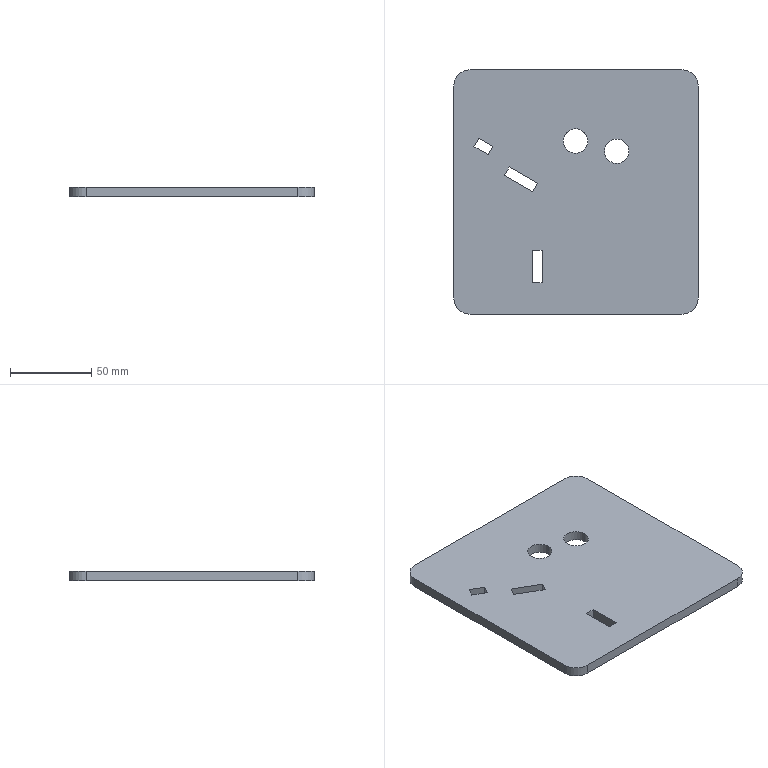Part | SolidWorks | features FlatPattern 1, SMBaseFlange 1, SheetMetal 1 | 1 solid | 26 faces | box 150 x 150 x 6 mm | volume 130564 mm3 | plane 18 | cylinder 8 | commonest cylinder face diameters 15 x4 20 x4
STEP:
#1=CARTESIAN_POINT('',(-26.981,-17.057,6.));
#2=VERTEX_POINT('',#1);
#3=CARTESIAN_POINT('',(-11.981,-17.057,6.));
#4=VERTEX_POINT('',#3);
#5=CARTESIAN_POINT('',(-19.481,-17.057,6.));
#6=DIRECTION('',(0.,0.,1.));
#7=DIRECTION('',(1.,0.,0.));
#8=AXIS2_PLACEMENT_3D('',#5,#6,#7);
#9=CIRCLE('',#8,7.5);
#10=EDGE_CURVE('',#2,#4,#9,.T.);
#11=ORIENTED_EDGE('',*,*,#10,.T.);
#12=CARTESIAN_POINT('',(-11.981,-17.057,0.));
#13=VERTEX_POINT('',#12);
#14=CARTESIAN_POINT('',(-11.981,-17.057,6.));
#15=DIRECTION('',(0.,0.,-1.));
#16=VECTOR('',#15,1000.);
#17=LINE('',#14,#16);
#18=EDGE_CURVE('',#4,#13,#17,.T.);
#19=ORIENTED_EDGE('',*,*,#18,.T.);
#20=CARTESIAN_POINT('',(-26.981,-17.057,0.));
#21=VERTEX_POINT('',#20);
#22=CARTESIAN_POINT('',(-19.481,-17.057,0.));
#23=DIRECTION('',(0.,0.,1.));
#24=DIRECTION('',(1.,0.,0.));
#25=AXIS2_PLACEMENT_3D('',#22,#23,#24);
#26=CIRCLE('',#25,7.5);
#27=EDGE_CURVE('',#21,#13,#26,.T.);
#28=ORIENTED_EDGE('',*,*,#27,.F.);
#29=CARTESIAN_POINT('',(-26.981,-17.057,6.));
#30=DIRECTION('',(0.,0.,-1.));
#31=VECTOR('',#30,1000.);
#32=LINE('',#29,#31);
#33=EDGE_CURVE('',#2,#21,#32,.T.);
#34=ORIENTED_EDGE('',*,*,#33,.F.);
#35=EDGE_LOOP('',(#11,#19,#28,#34));
#36=FACE_OUTER_BOUND('',#35,.T.);
#37=CARTESIAN_POINT('',(-19.481,-17.057,6.));
#38=DIRECTION('',(0.,0.,-1.));
#39=DIRECTION('',(-1.,0.,0.));
#40=AXIS2_PLACEMENT_3D('',#37,#38,#39);
#41=CYLINDRICAL_SURFACE('',#40,7.5);
#42=ADVANCED_FACE('',(#36),#41,.F.);
#43=CARTESIAN_POINT('',(-1.739,-23.292,6.));
#44=VERTEX_POINT('',#43);
#45=CARTESIAN_POINT('',(13.261,-23.292,6.));
#46=VERTEX_POINT('',#45);
#47=CARTESIAN_POINT('',(5.761,-23.292,6.));
#48=DIRECTION('',(0.,0.,1.));
#49=DIRECTION('',(1.,0.,0.));
#50=AXIS2_PLACEMENT_3D('',#47,#48,#49);
#51=CIRCLE('',#50,7.5);
#52=EDGE_CURVE('',#44,#46,#51,.T.);
#53=ORIENTED_EDGE('',*,*,#52,.T.);
#54=CARTESIAN_POINT('',(13.261,-23.292,0.));
#55=VERTEX_POINT('',#54);
#56=CARTESIAN_POINT('',(13.261,-23.292,6.));
#57=DIRECTION('',(0.,0.,-1.));
#58=VECTOR('',#57,1000.);
#59=LINE('',#56,#58);
#60=EDGE_CURVE('',#46,#55,#59,.T.);
#61=ORIENTED_EDGE('',*,*,#60,.T.);
#62=CARTESIAN_POINT('',(-1.739,-23.292,0.));
#63=VERTEX_POINT('',#62);
#64=CARTESIAN_POINT('',(5.761,-23.292,0.));
#65=DIRECTION('',(0.,0.,1.));
#66=DIRECTION('',(1.,0.,0.));
#67=AXIS2_PLACEMENT_3D('',#64,#65,#66);
#68=CIRCLE('',#67,7.5);
#69=EDGE_CURVE('',#63,#55,#68,.T.);
#70=ORIENTED_EDGE('',*,*,#69,.F.);
#71=CARTESIAN_POINT('',(-1.739,-23.292,6.));
#72=DIRECTION('',(0.,0.,-1.));
#73=VECTOR('',#72,1000.);
#74=LINE('',#71,#73);
#75=EDGE_CURVE('',#44,#63,#74,.T.);
#76=ORIENTED_EDGE('',*,*,#75,.F.);
#77=EDGE_LOOP('',(#53,#61,#70,#76));
#78=FACE_OUTER_BOUND('',#77,.T.);
#79=CARTESIAN_POINT('',(5.761,-23.292,6.));
#80=DIRECTION('',(0.,0.,-1.));
#81=DIRECTION('',(-1.,0.,0.));
#82=AXIS2_PLACEMENT_3D('',#79,#80,#81);
#83=CYLINDRICAL_SURFACE('',#82,7.5);
#84=ADVANCED_FACE('',(#78),#83,.F.);
#85=CARTESIAN_POINT('',(-45.869,-48.093,6.));
#86=VERTEX_POINT('',#85);
#87=CARTESIAN_POINT('',(-42.869,-42.897,6.));
#88=VERTEX_POINT('',#87);
#89=CARTESIAN_POINT('',(-45.869,-48.093,6.));
#90=DIRECTION('',(0.5,0.866,0.));
#91=VECTOR('',#90,1000.);
#92=LINE('',#89,#91);
#93=EDGE_CURVE('',#86,#88,#92,.T.);
#94=ORIENTED_EDGE('',*,*,#93,.F.);
#95=CARTESIAN_POINT('',(-63.19,-38.093,6.));
#96=VERTEX_POINT('',#95);
#97=CARTESIAN_POINT('',(-63.19,-38.093,6.));
#98=DIRECTION('',(0.866,-0.5,0.));
#99=VECTOR('',#98,1000.);
#100=LINE('',#97,#99);
#101=EDGE_CURVE('',#96,#86,#100,.T.);
#102=ORIENTED_EDGE('',*,*,#101,.F.);
#103=CARTESIAN_POINT('',(-60.19,-32.897,6.));
#104=VERTEX_POINT('',#103);
#105=CARTESIAN_POINT('',(-60.19,-32.897,6.));
#106=DIRECTION('',(-0.5,-0.866,0.));
#107=VECTOR('',#106,1000.);
#108=LINE('',#105,#107);
#109=EDGE_CURVE('',#104,#96,#108,.T.);
#110=ORIENTED_EDGE('',*,*,#109,.F.);
#111=CARTESIAN_POINT('',(-42.869,-42.897,6.));
#112=DIRECTION('',(-0.866,0.5,0.));
#113=VECTOR('',#112,1000.);
#114=LINE('',#111,#113);
#115=EDGE_CURVE('',#88,#104,#114,.T.);
#116=ORIENTED_EDGE('',*,*,#115,.F.);
#117=EDGE_LOOP('',(#94,#102,#110,#116));
#118=FACE_BOUND('',#117,.T.);
#119=ORIENTED_EDGE('',*,*,#10,.F.);
#120=CARTESIAN_POINT('',(-19.481,-17.057,6.));
#121=DIRECTION('',(0.,0.,1.));
#122=DIRECTION('',(1.,0.,0.));
#123=AXIS2_PLACEMENT_3D('',#120,#121,#122);
#124=CIRCLE('',#123,7.5);
#125=EDGE_CURVE('',#4,#2,#124,.T.);
#126=ORIENTED_EDGE('',*,*,#125,.F.);
#127=EDGE_LOOP('',(#119,#126));
#128=FACE_BOUND('',#127,.T.);
#129=ORIENTED_EDGE('',*,*,#52,.F.);
#130=CARTESIAN_POINT('',(5.761,-23.292,6.));
#131=DIRECTION('',(0.,0.,1.));
#132=DIRECTION('',(1.,0.,0.));
#133=AXIS2_PLACEMENT_3D('',#130,#131,#132);
#134=CIRCLE('',#133,7.5);
#135=EDGE_CURVE('',#46,#44,#134,.T.);
#136=ORIENTED_EDGE('',*,*,#135,.F.);
#137=EDGE_LOOP('',(#129,#136));
#138=FACE_BOUND('',#137,.T.);
#139=CARTESIAN_POINT('',(-84.239,26.708,6.));
#140=VERTEX_POINT('',#139);
#141=CARTESIAN_POINT('',(-94.239,16.708,6.));
#142=VERTEX_POINT('',#141);
#143=CARTESIAN_POINT('',(-84.239,16.708,6.));
#144=DIRECTION('',(0.,0.,1.));
#145=DIRECTION('',(-1.,0.,0.));
#146=AXIS2_PLACEMENT_3D('',#143,#144,#145);
#147=CIRCLE('',#146,10.);
#148=EDGE_CURVE('',#140,#142,#147,.T.);
#149=ORIENTED_EDGE('',*,*,#148,.T.);
#150=CARTESIAN_POINT('',(-94.239,-113.292,6.));
#151=VERTEX_POINT('',#150);
#152=CARTESIAN_POINT('',(-94.239,-113.292,6.));
#153=DIRECTION('',(0.,-1.,0.));
#154=VECTOR('',#153,1000.);
#155=LINE('',#152,#154);
#156=EDGE_CURVE('',#142,#151,#155,.T.);
#157=ORIENTED_EDGE('',*,*,#156,.T.);
#158=CARTESIAN_POINT('',(-84.239,-123.292,6.));
#159=VERTEX_POINT('',#158);
#160=CARTESIAN_POINT('',(-84.239,-113.292,6.));
#161=DIRECTION('',(0.,0.,1.));
#162=DIRECTION('',(-1.,0.,0.));
#163=AXIS2_PLACEMENT_3D('',#160,#161,#162);
#164=CIRCLE('',#163,10.);
#165=EDGE_CURVE('',#151,#159,#164,.T.);
#166=ORIENTED_EDGE('',*,*,#165,.T.);
#167=CARTESIAN_POINT('',(45.761,-123.292,6.));
#168=VERTEX_POINT('',#167);
#169=CARTESIAN_POINT('',(45.761,-123.292,6.));
#170=DIRECTION('',(1.,0.,0.));
#171=VECTOR('',#170,1000.);
#172=LINE('',#169,#171);
#173=EDGE_CURVE('',#159,#168,#172,.T.);
#174=ORIENTED_EDGE('',*,*,#173,.T.);
#175=CARTESIAN_POINT('',(55.761,-113.292,6.));
#176=VERTEX_POINT('',#175);
#177=CARTESIAN_POINT('',(45.761,-113.292,6.));
#178=DIRECTION('',(0.,0.,1.));
#179=DIRECTION('',(1.,0.,0.));
#180=AXIS2_PLACEMENT_3D('',#177,#178,#179);
#181=CIRCLE('',#180,10.);
#182=EDGE_CURVE('',#168,#176,#181,.T.);
#183=ORIENTED_EDGE('',*,*,#182,.T.);
#184=CARTESIAN_POINT('',(55.761,16.708,6.));
#185=VERTEX_POINT('',#184);
#186=CARTESIAN_POINT('',(55.761,16.708,6.));
#187=DIRECTION('',(0.,1.,0.));
#188=VECTOR('',#187,1000.);
#189=LINE('',#186,#188);
#190=EDGE_CURVE('',#176,#185,#189,.T.);
#191=ORIENTED_EDGE('',*,*,#190,.T.);
#192=CARTESIAN_POINT('',(45.761,26.708,6.));
#193=VERTEX_POINT('',#192);
#194=CARTESIAN_POINT('',(45.761,16.708,6.));
#195=DIRECTION('',(0.,0.,1.));
#196=DIRECTION('',(-1.,0.,0.));
#197=AXIS2_PLACEMENT_3D('',#194,#195,#196);
#198=CIRCLE('',#197,10.);
#199=EDGE_CURVE('',#185,#193,#198,.T.);
#200=ORIENTED_EDGE('',*,*,#199,.T.);
#201=CARTESIAN_POINT('',(-84.239,26.708,6.));
#202=DIRECTION('',(-1.,0.,0.));
#203=VECTOR('',#202,1000.);
#204=LINE('',#201,#203);
#205=EDGE_CURVE('',#193,#140,#204,.T.);
#206=ORIENTED_EDGE('',*,*,#205,.T.);
#207=EDGE_LOOP('',(#149,#157,#166,#174,#183,#191,#200,#206));
#208=FACE_OUTER_BOUND('',#207,.T.);
#209=CARTESIAN_POINT('',(-40.,-104.,6.));
#210=VERTEX_POINT('',#209);
#211=CARTESIAN_POINT('',(-40.,-84.,6.));
#212=VERTEX_POINT('',#211);
#213=CARTESIAN_POINT('',(-40.,-104.,6.));
#214=DIRECTION('',(0.,1.,0.));
#215=VECTOR('',#214,1000.);
#216=LINE('',#213,#215);
#217=EDGE_CURVE('',#210,#212,#216,.T.);
#218=ORIENTED_EDGE('',*,*,#217,.F.);
#219=CARTESIAN_POINT('',(-46.,-104.,6.));
#220=VERTEX_POINT('',#219);
#221=CARTESIAN_POINT('',(-46.,-104.,6.));
#222=DIRECTION('',(1.,0.,0.));
#223=VECTOR('',#222,1000.);
#224=LINE('',#221,#223);
#225=EDGE_CURVE('',#220,#210,#224,.T.);
#226=ORIENTED_EDGE('',*,*,#225,.F.);
#227=CARTESIAN_POINT('',(-46.,-84.,6.));
#228=VERTEX_POINT('',#227);
#229=CARTESIAN_POINT('',(-46.,-84.,6.));
#230=DIRECTION('',(0.,-1.,0.));
#231=VECTOR('',#230,1000.);
#232=LINE('',#229,#231);
#233=EDGE_CURVE('',#228,#220,#232,.T.);
#234=ORIENTED_EDGE('',*,*,#233,.F.);
#235=CARTESIAN_POINT('',(-40.,-84.,6.));
#236=DIRECTION('',(-1.,0.,0.));
#237=VECTOR('',#236,1000.);
#238=LINE('',#235,#237);
#239=EDGE_CURVE('',#212,#228,#238,.T.);
#240=ORIENTED_EDGE('',*,*,#239,.F.);
#241=EDGE_LOOP('',(#218,#226,#234,#240));
#242=FACE_BOUND('',#241,.T.);
#243=CARTESIAN_POINT('',(-78.84,-15.201,6.));
#244=VERTEX_POINT('',#243);
#245=CARTESIAN_POINT('',(-81.84,-20.397,6.));
#246=VERTEX_POINT('',#245);
#247=CARTESIAN_POINT('',(-81.84,-20.397,6.));
#248=DIRECTION('',(-0.5,-0.866,0.));
#249=VECTOR('',#248,1000.);
#250=LINE('',#247,#249);
#251=EDGE_CURVE('',#244,#246,#250,.T.);
#252=ORIENTED_EDGE('',*,*,#251,.F.);
#253=CARTESIAN_POINT('',(-70.18,-20.201,6.));
#254=VERTEX_POINT('',#253);
#255=CARTESIAN_POINT('',(-70.18,-20.201,6.));
#256=DIRECTION('',(-0.866,0.5,0.));
#257=VECTOR('',#256,1000.);
#258=LINE('',#255,#257);
#259=EDGE_CURVE('',#254,#244,#258,.T.);
#260=ORIENTED_EDGE('',*,*,#259,.F.);
#261=CARTESIAN_POINT('',(-73.18,-25.397,6.));
#262=VERTEX_POINT('',#261);
#263=CARTESIAN_POINT('',(-70.18,-20.201,6.));
#264=DIRECTION('',(0.5,0.866,0.));
#265=VECTOR('',#264,1000.);
#266=LINE('',#263,#265);
#267=EDGE_CURVE('',#262,#254,#266,.T.);
#268=ORIENTED_EDGE('',*,*,#267,.F.);
#269=CARTESIAN_POINT('',(-73.18,-25.397,6.));
#270=DIRECTION('',(0.866,-0.5,0.));
#271=VECTOR('',#270,1000.);
#272=LINE('',#269,#271);
#273=EDGE_CURVE('',#246,#262,#272,.T.);
#274=ORIENTED_EDGE('',*,*,#273,.F.);
#275=EDGE_LOOP('',(#252,#260,#268,#274));
#276=FACE_BOUND('',#275,.T.);
#277=CARTESIAN_POINT('',(-84.239,16.708,6.));
#278=DIRECTION('',(0.,0.,-1.));
#279=DIRECTION('',(-1.,0.,0.));
#280=AXIS2_PLACEMENT_3D('',#277,#278,#279);
#281=PLANE('',#280);
#282=ADVANCED_FACE('',(#118,#128,#138,#208,#242,#276),#281,.F.);
#283=ORIENTED_EDGE('',*,*,#69,.T.);
#284=CARTESIAN_POINT('',(5.761,-23.292,0.));
#285=DIRECTION('',(0.,0.,1.));
#286=DIRECTION('',(1.,0.,0.));
#287=AXIS2_PLACEMENT_3D('',#284,#285,#286);
#288=CIRCLE('',#287,7.5);
#289=EDGE_CURVE('',#55,#63,#288,.T.);
#290=ORIENTED_EDGE('',*,*,#289,.T.);
#291=EDGE_LOOP('',(#283,#290));
#292=FACE_BOUND('',#291,.T.);
#293=CARTESIAN_POINT('',(-84.239,26.708,0.));
#294=VERTEX_POINT('',#293);
#295=CARTESIAN_POINT('',(-94.239,16.708,0.));
#296=VERTEX_POINT('',#295);
#297=CARTESIAN_POINT('',(-84.239,16.708,0.));
#298=DIRECTION('',(0.,0.,1.));
#299=DIRECTION('',(-1.,0.,0.));
#300=AXIS2_PLACEMENT_3D('',#297,#298,#299);
#301=CIRCLE('',#300,10.);
#302=EDGE_CURVE('',#294,#296,#301,.T.);
#303=ORIENTED_EDGE('',*,*,#302,.F.);
#304=CARTESIAN_POINT('',(45.761,26.708,0.));
#305=VERTEX_POINT('',#304);
#306=CARTESIAN_POINT('',(-84.239,26.708,0.));
#307=DIRECTION('',(-1.,0.,0.));
#308=VECTOR('',#307,1000.);
#309=LINE('',#306,#308);
#310=EDGE_CURVE('',#305,#294,#309,.T.);
#311=ORIENTED_EDGE('',*,*,#310,.F.);
#312=CARTESIAN_POINT('',(55.761,16.708,0.));
#313=VERTEX_POINT('',#312);
#314=CARTESIAN_POINT('',(45.761,16.708,0.));
#315=DIRECTION('',(0.,0.,1.));
#316=DIRECTION('',(-1.,0.,0.));
#317=AXIS2_PLACEMENT_3D('',#314,#315,#316);
#318=CIRCLE('',#317,10.);
#319=EDGE_CURVE('',#313,#305,#318,.T.);
#320=ORIENTED_EDGE('',*,*,#319,.F.);
#321=CARTESIAN_POINT('',(55.761,-113.292,0.));
#322=VERTEX_POINT('',#321);
#323=CARTESIAN_POINT('',(55.761,16.708,0.));
#324=DIRECTION('',(0.,1.,0.));
#325=VECTOR('',#324,1000.);
#326=LINE('',#323,#325);
#327=EDGE_CURVE('',#322,#313,#326,.T.);
#328=ORIENTED_EDGE('',*,*,#327,.F.);
#329=CARTESIAN_POINT('',(45.761,-123.292,0.));
#330=VERTEX_POINT('',#329);
#331=CARTESIAN_POINT('',(45.761,-113.292,0.));
#332=DIRECTION('',(0.,0.,1.));
#333=DIRECTION('',(1.,0.,0.));
#334=AXIS2_PLACEMENT_3D('',#331,#332,#333);
#335=CIRCLE('',#334,10.);
#336=EDGE_CURVE('',#330,#322,#335,.T.);
#337=ORIENTED_EDGE('',*,*,#336,.F.);
#338=CARTESIAN_POINT('',(-84.239,-123.292,0.));
#339=VERTEX_POINT('',#338);
#340=CARTESIAN_POINT('',(45.761,-123.292,0.));
#341=DIRECTION('',(1.,0.,0.));
#342=VECTOR('',#341,1000.);
#343=LINE('',#340,#342);
#344=EDGE_CURVE('',#339,#330,#343,.T.);
#345=ORIENTED_EDGE('',*,*,#344,.F.);
#346=CARTESIAN_POINT('',(-94.239,-113.292,0.));
#347=VERTEX_POINT('',#346);
#348=CARTESIAN_POINT('',(-84.239,-113.292,0.));
#349=DIRECTION('',(0.,0.,1.));
#350=DIRECTION('',(-1.,0.,0.));
#351=AXIS2_PLACEMENT_3D('',#348,#349,#350);
#352=CIRCLE('',#351,10.);
#353=EDGE_CURVE('',#347,#339,#352,.T.);
#354=ORIENTED_EDGE('',*,*,#353,.F.);
#355=CARTESIAN_POINT('',(-94.239,-113.292,0.));
#356=DIRECTION('',(0.,-1.,0.));
#357=VECTOR('',#356,1000.);
#358=LINE('',#355,#357);
#359=EDGE_CURVE('',#296,#347,#358,.T.);
#360=ORIENTED_EDGE('',*,*,#359,.F.);
#361=EDGE_LOOP('',(#303,#311,#320,#328,#337,#345,#354,#360));
#362=FACE_OUTER_BOUND('',#361,.T.);
#363=ORIENTED_EDGE('',*,*,#27,.T.);
#364=CARTESIAN_POINT('',(-19.481,-17.057,0.));
#365=DIRECTION('',(0.,0.,1.));
#366=DIRECTION('',(1.,0.,0.));
#367=AXIS2_PLACEMENT_3D('',#364,#365,#366);
#368=CIRCLE('',#367,7.5);
#369=EDGE_CURVE('',#13,#21,#368,.T.);
#370=ORIENTED_EDGE('',*,*,#369,.T.);
#371=EDGE_LOOP('',(#363,#370));
#372=FACE_BOUND('',#371,.T.);
#373=CARTESIAN_POINT('',(-46.,-104.,0.));
#374=VERTEX_POINT('',#373);
#375=CARTESIAN_POINT('',(-40.,-104.,0.));
#376=VERTEX_POINT('',#375);
#377=CARTESIAN_POINT('',(-46.,-104.,0.));
#378=DIRECTION('',(1.,0.,0.));
#379=VECTOR('',#378,1000.);
#380=LINE('',#377,#379);
#381=EDGE_CURVE('',#374,#376,#380,.T.);
#382=ORIENTED_EDGE('',*,*,#381,.T.);
#383=CARTESIAN_POINT('',(-40.,-84.,0.));
#384=VERTEX_POINT('',#383);
#385=CARTESIAN_POINT('',(-40.,-104.,0.));
#386=DIRECTION('',(0.,1.,0.));
#387=VECTOR('',#386,1000.);
#388=LINE('',#385,#387);
#389=EDGE_CURVE('',#376,#384,#388,.T.);
#390=ORIENTED_EDGE('',*,*,#389,.T.);
#391=CARTESIAN_POINT('',(-46.,-84.,0.));
#392=VERTEX_POINT('',#391);
#393=CARTESIAN_POINT('',(-40.,-84.,0.));
#394=DIRECTION('',(-1.,0.,0.));
#395=VECTOR('',#394,1000.);
#396=LINE('',#393,#395);
#397=EDGE_CURVE('',#384,#392,#396,.T.);
#398=ORIENTED_EDGE('',*,*,#397,.T.);
#399=CARTESIAN_POINT('',(-46.,-84.,0.));
#400=DIRECTION('',(0.,-1.,0.));
#401=VECTOR('',#400,1000.);
#402=LINE('',#399,#401);
#403=EDGE_CURVE('',#392,#374,#402,.T.);
#404=ORIENTED_EDGE('',*,*,#403,.T.);
#405=EDGE_LOOP('',(#382,#390,#398,#404));
#406=FACE_BOUND('',#405,.T.);
#407=CARTESIAN_POINT('',(-63.19,-38.093,0.));
#408=VERTEX_POINT('',#407);
#409=CARTESIAN_POINT('',(-45.869,-48.093,0.));
#410=VERTEX_POINT('',#409);
#411=CARTESIAN_POINT('',(-63.19,-38.093,0.));
#412=DIRECTION('',(0.866,-0.5,0.));
#413=VECTOR('',#412,1000.);
#414=LINE('',#411,#413);
#415=EDGE_CURVE('',#408,#410,#414,.T.);
#416=ORIENTED_EDGE('',*,*,#415,.T.);
#417=CARTESIAN_POINT('',(-42.869,-42.897,0.));
#418=VERTEX_POINT('',#417);
#419=CARTESIAN_POINT('',(-45.869,-48.093,0.));
#420=DIRECTION('',(0.5,0.866,0.));
#421=VECTOR('',#420,1000.);
#422=LINE('',#419,#421);
#423=EDGE_CURVE('',#410,#418,#422,.T.);
#424=ORIENTED_EDGE('',*,*,#423,.T.);
#425=CARTESIAN_POINT('',(-60.19,-32.897,0.));
#426=VERTEX_POINT('',#425);
#427=CARTESIAN_POINT('',(-42.869,-42.897,0.));
#428=DIRECTION('',(-0.866,0.5,0.));
#429=VECTOR('',#428,1000.);
#430=LINE('',#427,#429);
#431=EDGE_CURVE('',#418,#426,#430,.T.);
#432=ORIENTED_EDGE('',*,*,#431,.T.);
#433=CARTESIAN_POINT('',(-60.19,-32.897,0.));
#434=DIRECTION('',(-0.5,-0.866,0.));
#435=VECTOR('',#434,1000.);
#436=LINE('',#433,#435);
#437=EDGE_CURVE('',#426,#408,#436,.T.);
#438=ORIENTED_EDGE('',*,*,#437,.T.);
#439=EDGE_LOOP('',(#416,#424,#432,#438));
#440=FACE_BOUND('',#439,.T.);
#441=CARTESIAN_POINT('',(-70.18,-20.201,0.));
#442=VERTEX_POINT('',#441);
#443=CARTESIAN_POINT('',(-78.84,-15.201,0.));
#444=VERTEX_POINT('',#443);
#445=CARTESIAN_POINT('',(-70.18,-20.201,0.));
#446=DIRECTION('',(-0.866,0.5,0.));
#447=VECTOR('',#446,1000.);
#448=LINE('',#445,#447);
#449=EDGE_CURVE('',#442,#444,#448,.T.);
#450=ORIENTED_EDGE('',*,*,#449,.T.);
#451=CARTESIAN_POINT('',(-81.84,-20.397,0.));
#452=VERTEX_POINT('',#451);
#453=CARTESIAN_POINT('',(-81.84,-20.397,0.));
#454=DIRECTION('',(-0.5,-0.866,0.));
#455=VECTOR('',#454,1000.);
#456=LINE('',#453,#455);
#457=EDGE_CURVE('',#444,#452,#456,.T.);
#458=ORIENTED_EDGE('',*,*,#457,.T.);
#459=CARTESIAN_POINT('',(-73.18,-25.397,0.));
#460=VERTEX_POINT('',#459);
#461=CARTESIAN_POINT('',(-73.18,-25.397,0.));
#462=DIRECTION('',(0.866,-0.5,0.));
#463=VECTOR('',#462,1000.);
#464=LINE('',#461,#463);
#465=EDGE_CURVE('',#452,#460,#464,.T.);
#466=ORIENTED_EDGE('',*,*,#465,.T.);
#467=CARTESIAN_POINT('',(-70.18,-20.201,0.));
#468=DIRECTION('',(0.5,0.866,0.));
#469=VECTOR('',#468,1000.);
#470=LINE('',#467,#469);
#471=EDGE_CURVE('',#460,#442,#470,.T.);
#472=ORIENTED_EDGE('',*,*,#471,.T.);
#473=EDGE_LOOP('',(#450,#458,#466,#472));
#474=FACE_BOUND('',#473,.T.);
#475=CARTESIAN_POINT('',(-84.239,16.708,0.));
#476=DIRECTION('',(0.,0.,-1.));
#477=DIRECTION('',(-1.,0.,0.));
#478=AXIS2_PLACEMENT_3D('',#475,#476,#477);
#479=PLANE('',#478);
#480=ADVANCED_FACE('',(#292,#362,#372,#406,#440,#474),#479,.T.);
#481=ORIENTED_EDGE('',*,*,#302,.T.);
#482=CARTESIAN_POINT('',(-94.239,16.708,6.));
#483=DIRECTION('',(0.,0.,-1.));
#484=VECTOR('',#483,1000.);
#485=LINE('',#482,#484);
#486=EDGE_CURVE('',#142,#296,#485,.T.);
#487=ORIENTED_EDGE('',*,*,#486,.F.);
#488=ORIENTED_EDGE('',*,*,#148,.F.);
#489=CARTESIAN_POINT('',(-84.239,26.708,6.));
#490=DIRECTION('',(0.,0.,-1.));
#491=VECTOR('',#490,1000.);
#492=LINE('',#489,#491);
#493=EDGE_CURVE('',#140,#294,#492,.T.);
#494=ORIENTED_EDGE('',*,*,#493,.T.);
#495=EDGE_LOOP('',(#481,#487,#488,#494));
#496=FACE_OUTER_BOUND('',#495,.T.);
#497=CARTESIAN_POINT('',(-84.239,16.708,6.));
#498=DIRECTION('',(0.,0.,-1.));
#499=DIRECTION('',(-1.,0.,0.));
#500=AXIS2_PLACEMENT_3D('',#497,#498,#499);
#501=CYLINDRICAL_SURFACE('',#500,10.);
#502=ADVANCED_FACE('',(#496),#501,.T.);
#503=ORIENTED_EDGE('',*,*,#359,.T.);
#504=CARTESIAN_POINT('',(-94.239,-113.292,6.));
#505=DIRECTION('',(0.,0.,-1.));
#506=VECTOR('',#505,1000.);
#507=LINE('',#504,#506);
#508=EDGE_CURVE('',#151,#347,#507,.T.);
#509=ORIENTED_EDGE('',*,*,#508,.F.);
#510=ORIENTED_EDGE('',*,*,#156,.F.);
#511=ORIENTED_EDGE('',*,*,#486,.T.);
#512=EDGE_LOOP('',(#503,#509,#510,#511));
#513=FACE_OUTER_BOUND('',#512,.T.);
#514=CARTESIAN_POINT('',(-94.239,-113.292,6.));
#515=DIRECTION('',(1.,0.,0.));
#516=DIRECTION('',(0.,1.,0.));
#517=AXIS2_PLACEMENT_3D('',#514,#515,#516);
#518=PLANE('',#517);
#519=ADVANCED_FACE('',(#513),#518,.F.);
#520=ORIENTED_EDGE('',*,*,#353,.T.);
#521=CARTESIAN_POINT('',(-84.239,-123.292,6.));
#522=DIRECTION('',(0.,0.,-1.));
#523=VECTOR('',#522,1000.);
#524=LINE('',#521,#523);
#525=EDGE_CURVE('',#159,#339,#524,.T.);
#526=ORIENTED_EDGE('',*,*,#525,.F.);
#527=ORIENTED_EDGE('',*,*,#165,.F.);
#528=ORIENTED_EDGE('',*,*,#508,.T.);
#529=EDGE_LOOP('',(#520,#526,#527,#528));
#530=FACE_OUTER_BOUND('',#529,.T.);
#531=CARTESIAN_POINT('',(-84.239,-113.292,6.));
#532=DIRECTION('',(0.,0.,-1.));
#533=DIRECTION('',(-1.,0.,0.));
#534=AXIS2_PLACEMENT_3D('',#531,#532,#533);
#535=CYLINDRICAL_SURFACE('',#534,10.);
#536=ADVANCED_FACE('',(#530),#535,.T.);
#537=ORIENTED_EDGE('',*,*,#344,.T.);
#538=CARTESIAN_POINT('',(45.761,-123.292,6.));
#539=DIRECTION('',(0.,0.,-1.));
#540=VECTOR('',#539,1000.);
#541=LINE('',#538,#540);
#542=EDGE_CURVE('',#168,#330,#541,.T.);
#543=ORIENTED_EDGE('',*,*,#542,.F.);
#544=ORIENTED_EDGE('',*,*,#173,.F.);
#545=ORIENTED_EDGE('',*,*,#525,.T.);
#546=EDGE_LOOP('',(#537,#543,#544,#545));
#547=FACE_OUTER_BOUND('',#546,.T.);
#548=CARTESIAN_POINT('',(45.761,-123.292,6.));
#549=DIRECTION('',(0.,1.,0.));
#550=DIRECTION('',(-1.,0.,0.));
#551=AXIS2_PLACEMENT_3D('',#548,#549,#550);
#552=PLANE('',#551);
#553=ADVANCED_FACE('',(#547),#552,.F.);
#554=ORIENTED_EDGE('',*,*,#336,.T.);
#555=CARTESIAN_POINT('',(55.761,-113.292,6.));
#556=DIRECTION('',(0.,0.,-1.));
#557=VECTOR('',#556,1000.);
#558=LINE('',#555,#557);
#559=EDGE_CURVE('',#176,#322,#558,.T.);
#560=ORIENTED_EDGE('',*,*,#559,.F.);
#561=ORIENTED_EDGE('',*,*,#182,.F.);
#562=ORIENTED_EDGE('',*,*,#542,.T.);
#563=EDGE_LOOP('',(#554,#560,#561,#562));
#564=FACE_OUTER_BOUND('',#563,.T.);
#565=CARTESIAN_POINT('',(45.761,-113.292,6.));
#566=DIRECTION('',(0.,0.,-1.));
#567=DIRECTION('',(-1.,0.,0.));
#568=AXIS2_PLACEMENT_3D('',#565,#566,#567);
#569=CYLINDRICAL_SURFACE('',#568,10.);
#570=ADVANCED_FACE('',(#564),#569,.T.);
#571=ORIENTED_EDGE('',*,*,#327,.T.);
#572=CARTESIAN_POINT('',(55.761,16.708,6.));
#573=DIRECTION('',(0.,0.,-1.));
#574=VECTOR('',#573,1000.);
#575=LINE('',#572,#574);
#576=EDGE_CURVE('',#185,#313,#575,.T.);
#577=ORIENTED_EDGE('',*,*,#576,.F.);
#578=ORIENTED_EDGE('',*,*,#190,.F.);
#579=ORIENTED_EDGE('',*,*,#559,.T.);
#580=EDGE_LOOP('',(#571,#577,#578,#579));
#581=FACE_OUTER_BOUND('',#580,.T.);
#582=CARTESIAN_POINT('',(55.761,16.708,6.));
#583=DIRECTION('',(-1.,0.,0.));
#584=DIRECTION('',(0.,-1.,0.));
#585=AXIS2_PLACEMENT_3D('',#582,#583,#584);
#586=PLANE('',#585);
#587=ADVANCED_FACE('',(#581),#586,.F.);
#588=ORIENTED_EDGE('',*,*,#319,.T.);
#589=CARTESIAN_POINT('',(45.761,26.708,6.));
#590=DIRECTION('',(0.,0.,-1.));
#591=VECTOR('',#590,1000.);
#592=LINE('',#589,#591);
#593=EDGE_CURVE('',#193,#305,#592,.T.);
#594=ORIENTED_EDGE('',*,*,#593,.F.);
#595=ORIENTED_EDGE('',*,*,#199,.F.);
#596=ORIENTED_EDGE('',*,*,#576,.T.);
#597=EDGE_LOOP('',(#588,#594,#595,#596));
#598=FACE_OUTER_BOUND('',#597,.T.);
#599=CARTESIAN_POINT('',(45.761,16.708,6.));
#600=DIRECTION('',(0.,0.,-1.));
#601=DIRECTION('',(-1.,0.,0.));
#602=AXIS2_PLACEMENT_3D('',#599,#600,#601);
#603=CYLINDRICAL_SURFACE('',#602,10.);
#604=ADVANCED_FACE('',(#598),#603,.T.);
#605=ORIENTED_EDGE('',*,*,#310,.T.);
#606=ORIENTED_EDGE('',*,*,#493,.F.);
#607=ORIENTED_EDGE('',*,*,#205,.F.);
#608=ORIENTED_EDGE('',*,*,#593,.T.);
#609=EDGE_LOOP('',(#605,#606,#607,#608));
#610=FACE_OUTER_BOUND('',#609,.T.);
#611=CARTESIAN_POINT('',(-84.239,26.708,6.));
#612=DIRECTION('',(0.,-1.,0.));
#613=DIRECTION('',(0.,0.,-1.));
#614=AXIS2_PLACEMENT_3D('',#611,#612,#613);
#615=PLANE('',#614);
#616=ADVANCED_FACE('',(#610),#615,.F.);
#617=ORIENTED_EDGE('',*,*,#60,.F.);
#618=ORIENTED_EDGE('',*,*,#135,.T.);
#619=ORIENTED_EDGE('',*,*,#75,.T.);
#620=ORIENTED_EDGE('',*,*,#289,.F.);
#621=EDGE_LOOP('',(#617,#618,#619,#620));
#622=FACE_OUTER_BOUND('',#621,.T.);
#623=CARTESIAN_POINT('',(5.761,-23.292,6.));
#624=DIRECTION('',(0.,0.,-1.));
#625=DIRECTION('',(-1.,0.,0.));
#626=AXIS2_PLACEMENT_3D('',#623,#624,#625);
#627=CYLINDRICAL_SURFACE('',#626,7.5);
#628=ADVANCED_FACE('',(#622),#627,.F.);
#629=ORIENTED_EDGE('',*,*,#18,.F.);
#630=ORIENTED_EDGE('',*,*,#125,.T.);
#631=ORIENTED_EDGE('',*,*,#33,.T.);
#632=ORIENTED_EDGE('',*,*,#369,.F.);
#633=EDGE_LOOP('',(#629,#630,#631,#632));
#634=FACE_OUTER_BOUND('',#633,.T.);
#635=CARTESIAN_POINT('',(-19.481,-17.057,6.));
#636=DIRECTION('',(0.,0.,-1.));
#637=DIRECTION('',(-1.,0.,0.));
#638=AXIS2_PLACEMENT_3D('',#635,#636,#637);
#639=CYLINDRICAL_SURFACE('',#638,7.5);
#640=ADVANCED_FACE('',(#634),#639,.F.);
#641=ORIENTED_EDGE('',*,*,#389,.F.);
#642=CARTESIAN_POINT('',(-40.,-104.,6.));
#643=DIRECTION('',(0.,0.,-1.));
#644=VECTOR('',#643,1000.);
#645=LINE('',#642,#644);
#646=EDGE_CURVE('',#210,#376,#645,.T.);
#647=ORIENTED_EDGE('',*,*,#646,.F.);
#648=ORIENTED_EDGE('',*,*,#217,.T.);
#649=CARTESIAN_POINT('',(-40.,-84.,6.));
#650=DIRECTION('',(0.,0.,-1.));
#651=VECTOR('',#650,1000.);
#652=LINE('',#649,#651);
#653=EDGE_CURVE('',#212,#384,#652,.T.);
#654=ORIENTED_EDGE('',*,*,#653,.T.);
#655=EDGE_LOOP('',(#641,#647,#648,#654));
#656=FACE_OUTER_BOUND('',#655,.T.);
#657=CARTESIAN_POINT('',(-40.,-104.,6.));
#658=DIRECTION('',(-1.,0.,0.));
#659=DIRECTION('',(0.,0.,1.));
#660=AXIS2_PLACEMENT_3D('',#657,#658,#659);
#661=PLANE('',#660);
#662=ADVANCED_FACE('',(#656),#661,.T.);
#663=ORIENTED_EDGE('',*,*,#397,.F.);
#664=ORIENTED_EDGE('',*,*,#653,.F.);
#665=ORIENTED_EDGE('',*,*,#239,.T.);
#666=CARTESIAN_POINT('',(-46.,-84.,6.));
#667=DIRECTION('',(0.,0.,-1.));
#668=VECTOR('',#667,1000.);
#669=LINE('',#666,#668);
#670=EDGE_CURVE('',#228,#392,#669,.T.);
#671=ORIENTED_EDGE('',*,*,#670,.T.);
#672=EDGE_LOOP('',(#663,#664,#665,#671));
#673=FACE_OUTER_BOUND('',#672,.T.);
#674=CARTESIAN_POINT('',(-40.,-84.,6.));
#675=DIRECTION('',(0.,-1.,0.));
#676=DIRECTION('',(0.,0.,-1.));
#677=AXIS2_PLACEMENT_3D('',#674,#675,#676);
#678=PLANE('',#677);
#679=ADVANCED_FACE('',(#673),#678,.T.);
#680=ORIENTED_EDGE('',*,*,#403,.F.);
#681=ORIENTED_EDGE('',*,*,#670,.F.);
#682=ORIENTED_EDGE('',*,*,#233,.T.);
#683=CARTESIAN_POINT('',(-46.,-104.,6.));
#684=DIRECTION('',(0.,0.,-1.));
#685=VECTOR('',#684,1000.);
#686=LINE('',#683,#685);
#687=EDGE_CURVE('',#220,#374,#686,.T.);
#688=ORIENTED_EDGE('',*,*,#687,.T.);
#689=EDGE_LOOP('',(#680,#681,#682,#688));
#690=FACE_OUTER_BOUND('',#689,.T.);
#691=CARTESIAN_POINT('',(-46.,-84.,6.));
#692=DIRECTION('',(1.,0.,0.));
#693=DIRECTION('',(0.,0.,-1.));
#694=AXIS2_PLACEMENT_3D('',#691,#692,#693);
#695=PLANE('',#694);
#696=ADVANCED_FACE('',(#690),#695,.T.);
#697=ORIENTED_EDGE('',*,*,#381,.F.);
#698=ORIENTED_EDGE('',*,*,#687,.F.);
#699=ORIENTED_EDGE('',*,*,#225,.T.);
#700=ORIENTED_EDGE('',*,*,#646,.T.);
#701=EDGE_LOOP('',(#697,#698,#699,#700));
#702=FACE_OUTER_BOUND('',#701,.T.);
#703=CARTESIAN_POINT('',(-46.,-104.,6.));
#704=DIRECTION('',(0.,1.,0.));
#705=DIRECTION('',(0.,0.,1.));
#706=AXIS2_PLACEMENT_3D('',#703,#704,#705);
#707=PLANE('',#706);
#708=ADVANCED_FACE('',(#702),#707,.T.);
#709=ORIENTED_EDGE('',*,*,#423,.F.);
#710=CARTESIAN_POINT('',(-45.869,-48.093,6.));
#711=DIRECTION('',(0.,0.,-1.));
#712=VECTOR('',#711,1000.);
#713=LINE('',#710,#712);
#714=EDGE_CURVE('',#86,#410,#713,.T.);
#715=ORIENTED_EDGE('',*,*,#714,.F.);
#716=ORIENTED_EDGE('',*,*,#93,.T.);
#717=CARTESIAN_POINT('',(-42.869,-42.897,6.));
#718=DIRECTION('',(0.,0.,-1.));
#719=VECTOR('',#718,1000.);
#720=LINE('',#717,#719);
#721=EDGE_CURVE('',#88,#418,#720,.T.);
#722=ORIENTED_EDGE('',*,*,#721,.T.);
#723=EDGE_LOOP('',(#709,#715,#716,#722));
#724=FACE_OUTER_BOUND('',#723,.T.);
#725=CARTESIAN_POINT('',(-45.869,-48.093,6.));
#726=DIRECTION('',(-0.866,0.5,0.));
#727=DIRECTION('',(-0.5,-0.866,0.));
#728=AXIS2_PLACEMENT_3D('',#725,#726,#727);
#729=PLANE('',#728);
#730=ADVANCED_FACE('',(#724),#729,.T.);
#731=ORIENTED_EDGE('',*,*,#431,.F.);
#732=ORIENTED_EDGE('',*,*,#721,.F.);
#733=ORIENTED_EDGE('',*,*,#115,.T.);
#734=CARTESIAN_POINT('',(-60.19,-32.897,6.));
#735=DIRECTION('',(0.,0.,-1.));
#736=VECTOR('',#735,1000.);
#737=LINE('',#734,#736);
#738=EDGE_CURVE('',#104,#426,#737,.T.);
#739=ORIENTED_EDGE('',*,*,#738,.T.);
#740=EDGE_LOOP('',(#731,#732,#733,#739));
#741=FACE_OUTER_BOUND('',#740,.T.);
#742=CARTESIAN_POINT('',(-42.869,-42.897,6.));
#743=DIRECTION('',(-0.5,-0.866,0.));
#744=DIRECTION('',(0.866,-0.5,0.));
#745=AXIS2_PLACEMENT_3D('',#742,#743,#744);
#746=PLANE('',#745);
#747=ADVANCED_FACE('',(#741),#746,.T.);
#748=ORIENTED_EDGE('',*,*,#437,.F.);
#749=ORIENTED_EDGE('',*,*,#738,.F.);
#750=ORIENTED_EDGE('',*,*,#109,.T.);
#751=CARTESIAN_POINT('',(-63.19,-38.093,6.));
#752=DIRECTION('',(0.,0.,-1.));
#753=VECTOR('',#752,1000.);
#754=LINE('',#751,#753);
#755=EDGE_CURVE('',#96,#408,#754,.T.);
#756=ORIENTED_EDGE('',*,*,#755,.T.);
#757=EDGE_LOOP('',(#748,#749,#750,#756));
#758=FACE_OUTER_BOUND('',#757,.T.);
#759=CARTESIAN_POINT('',(-60.19,-32.897,6.));
#760=DIRECTION('',(0.866,-0.5,0.));
#761=DIRECTION('',(0.5,0.866,0.));
#762=AXIS2_PLACEMENT_3D('',#759,#760,#761);
#763=PLANE('',#762);
#764=ADVANCED_FACE('',(#758),#763,.T.);
#765=ORIENTED_EDGE('',*,*,#415,.F.);
#766=ORIENTED_EDGE('',*,*,#755,.F.);
#767=ORIENTED_EDGE('',*,*,#101,.T.);
#768=ORIENTED_EDGE('',*,*,#714,.T.);
#769=EDGE_LOOP('',(#765,#766,#767,#768));
#770=FACE_OUTER_BOUND('',#769,.T.);
#771=CARTESIAN_POINT('',(-63.19,-38.093,6.));
#772=DIRECTION('',(0.5,0.866,0.));
#773=DIRECTION('',(-0.866,0.5,0.));
#774=AXIS2_PLACEMENT_3D('',#771,#772,#773);
#775=PLANE('',#774);
#776=ADVANCED_FACE('',(#770),#775,.T.);
#777=ORIENTED_EDGE('',*,*,#457,.F.);
#778=CARTESIAN_POINT('',(-78.84,-15.201,6.));
#779=DIRECTION('',(0.,0.,-1.));
#780=VECTOR('',#779,1000.);
#781=LINE('',#778,#780);
#782=EDGE_CURVE('',#244,#444,#781,.T.);
#783=ORIENTED_EDGE('',*,*,#782,.F.);
#784=ORIENTED_EDGE('',*,*,#251,.T.);
#785=CARTESIAN_POINT('',(-81.84,-20.397,6.));
#786=DIRECTION('',(0.,0.,-1.));
#787=VECTOR('',#786,1000.);
#788=LINE('',#785,#787);
#789=EDGE_CURVE('',#246,#452,#788,.T.);
#790=ORIENTED_EDGE('',*,*,#789,.T.);
#791=EDGE_LOOP('',(#777,#783,#784,#790));
#792=FACE_OUTER_BOUND('',#791,.T.);
#793=CARTESIAN_POINT('',(-81.84,-20.397,6.));
#794=DIRECTION('',(0.866,-0.5,0.));
#795=DIRECTION('',(0.5,0.866,0.));
#796=AXIS2_PLACEMENT_3D('',#793,#794,#795);
#797=PLANE('',#796);
#798=ADVANCED_FACE('',(#792),#797,.T.);
#799=ORIENTED_EDGE('',*,*,#465,.F.);
#800=ORIENTED_EDGE('',*,*,#789,.F.);
#801=ORIENTED_EDGE('',*,*,#273,.T.);
#802=CARTESIAN_POINT('',(-73.18,-25.397,6.));
#803=DIRECTION('',(0.,0.,-1.));
#804=VECTOR('',#803,1000.);
#805=LINE('',#802,#804);
#806=EDGE_CURVE('',#262,#460,#805,.T.);
#807=ORIENTED_EDGE('',*,*,#806,.T.);
#808=EDGE_LOOP('',(#799,#800,#801,#807));
#809=FACE_OUTER_BOUND('',#808,.T.);
#810=CARTESIAN_POINT('',(-73.18,-25.397,6.));
#811=DIRECTION('',(0.5,0.866,0.));
#812=DIRECTION('',(-0.866,0.5,0.));
#813=AXIS2_PLACEMENT_3D('',#810,#811,#812);
#814=PLANE('',#813);
#815=ADVANCED_FACE('',(#809),#814,.T.);
#816=ORIENTED_EDGE('',*,*,#471,.F.);
#817=ORIENTED_EDGE('',*,*,#806,.F.);
#818=ORIENTED_EDGE('',*,*,#267,.T.);
#819=CARTESIAN_POINT('',(-70.18,-20.201,6.));
#820=DIRECTION('',(0.,0.,-1.));
#821=VECTOR('',#820,1000.);
#822=LINE('',#819,#821);
#823=EDGE_CURVE('',#254,#442,#822,.T.);
#824=ORIENTED_EDGE('',*,*,#823,.T.);
#825=EDGE_LOOP('',(#816,#817,#818,#824));
#826=FACE_OUTER_BOUND('',#825,.T.);
#827=CARTESIAN_POINT('',(-70.18,-20.201,6.));
#828=DIRECTION('',(-0.866,0.5,0.));
#829=DIRECTION('',(-0.5,-0.866,0.));
#830=AXIS2_PLACEMENT_3D('',#827,#828,#829);
#831=PLANE('',#830);
#832=ADVANCED_FACE('',(#826),#831,.T.);
#833=ORIENTED_EDGE('',*,*,#449,.F.);
#834=ORIENTED_EDGE('',*,*,#823,.F.);
#835=ORIENTED_EDGE('',*,*,#259,.T.);
#836=ORIENTED_EDGE('',*,*,#782,.T.);
#837=EDGE_LOOP('',(#833,#834,#835,#836));
#838=FACE_OUTER_BOUND('',#837,.T.);
#839=CARTESIAN_POINT('',(-70.18,-20.201,6.));
#840=DIRECTION('',(-0.5,-0.866,0.));
#841=DIRECTION('',(0.866,-0.5,0.));
#842=AXIS2_PLACEMENT_3D('',#839,#840,#841);
#843=PLANE('',#842);
#844=ADVANCED_FACE('',(#838),#843,.T.);
#845=CLOSED_SHELL('',(#42,#84,#282,#480,#502,#519,#536,#553,#570,#587,#604,#616,#628,#640,#662,#679,#696,#708,#730,#747,#764,#776,#798,#815,#832,#844));
#846=MANIFOLD_SOLID_BREP('',#845);
#847=CARTESIAN_POINT('',(0.,0.,0.));
#848=DIRECTION('',(0.,0.,1.));
#849=DIRECTION('',(1.,0.,0.));
#850=AXIS2_PLACEMENT_3D('',#847,#848,#849);
#851=(LENGTH_UNIT()NAMED_UNIT(*)SI_UNIT(.MILLI.,.METRE.));
#852=UNCERTAINTY_MEASURE_WITH_UNIT(LENGTH_MEASURE(0.00001),#851,'','');
#853=(NAMED_UNIT(*)PLANE_ANGLE_UNIT()SI_UNIT($,.RADIAN.));
#854=(NAMED_UNIT(*)SI_UNIT($,.STERADIAN.)SOLID_ANGLE_UNIT());
#855=(GEOMETRIC_REPRESENTATION_CONTEXT(3)GLOBAL_UNCERTAINTY_ASSIGNED_CONTEXT((#852))GLOBAL_UNIT_ASSIGNED_CONTEXT((#851,#853,#854))REPRESENTATION_CONTEXT('',''));
#856=ADVANCED_BREP_SHAPE_REPRESENTATION('',(#846,#850),#855);